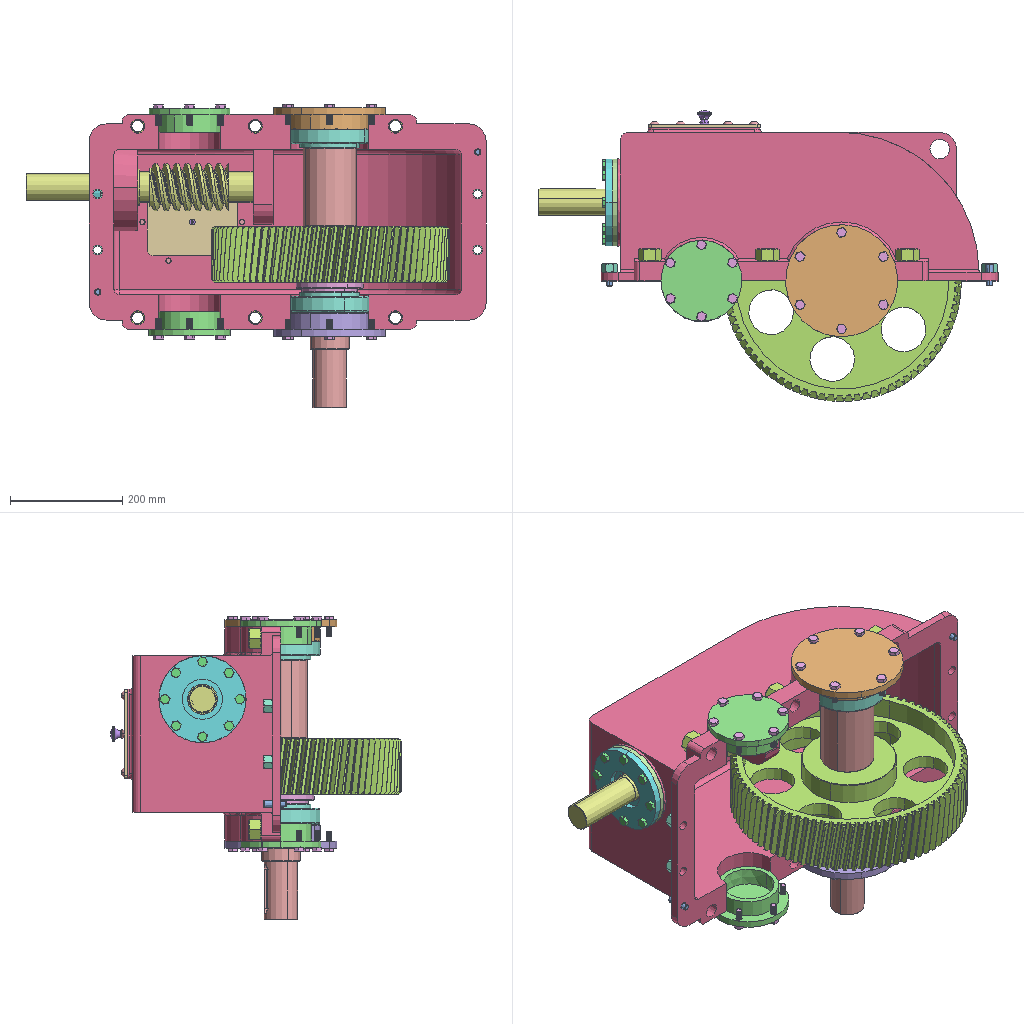Assembly | SolidWorks | 38 different items | 97 placed | box 821 x 519 x 542 mm
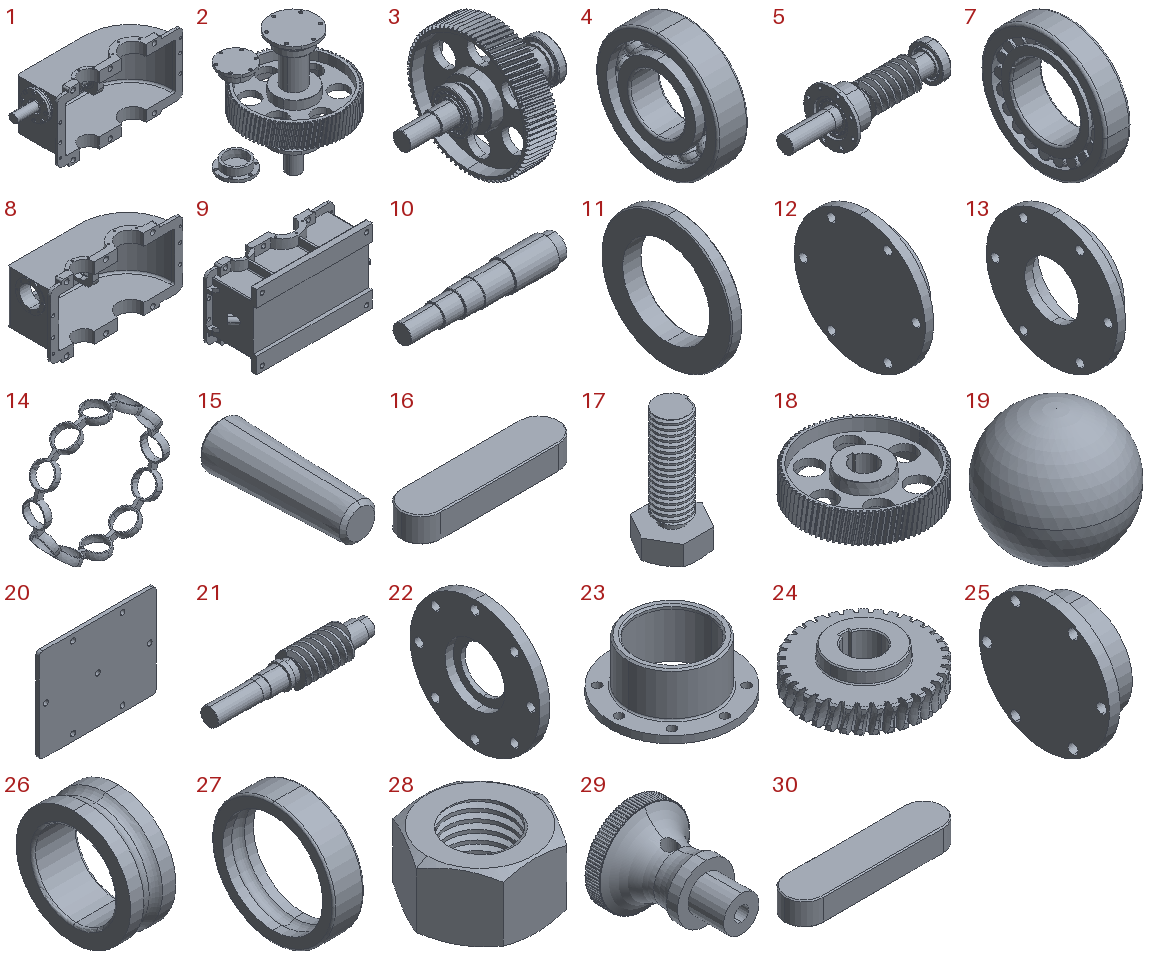Parts list (item | name | quantity | parent item | size | volume | features):
1 | (subassembly) | x1 | - | 820.75 x 304 x 382 mm | 10937552 mm3 | features CompositeCurve 13
2 | (subassembly) | x1 | - | 535.812 x 424.15 x 535.75 mm | 9344461 mm3 | -
3 | (subassembly) | x1 | in 2 | 499.25 x 424.15 x 424.15 mm | 7884570 mm3 | -
4 | (subassembly) | x1 | in 5 | 25 x 100 x 100 mm | 114868 mm3 | features ReferencePattern 11, LocalCirPattern 1
5 | (subassembly) | x1 | in 1 | 432 x 156 x 156 mm | 1680982 mm3 | -
6 | (subassembly) | x1 | - | - | - | -
7 | - | x4 | in 3, 5 | 26.75 x 100 x 100 mm | 98923 mm3 | features Revolution 3, CirPattern 1
8 | - | x1 | in 1 | 708 x 273 x 382 mm | 8807514 mm3 | features ICE 13, Fillet 10, HoleWzd 5, MirrorPattern 4, 3DProfileFeature 2, CirPattern 1, Extrusion 1, RevCut 1, Shell 1
9 | - | x1 | - | 708.739 x 260 x 410 mm | 11835781 mm3 | features ICE 11, MirrorPattern 5, Fillet 4, HoleWzd 4, CirPattern 3, Rib 2, Extrusion 1, LPattern 1
10 | - | x1 | in 3 | 497 x 95 x 95 mm | 2516140 mm3 | features ICE 2, Chamfer 1, Fillet 1, Revolution 1
11 | - | x1 | in 3 | 17.75 x 120 x 120 mm | 86679 mm3 | features Chamfer 1, Revolution 1
12 | - | x1 | in 2 | 38.75 x 200 x 200 mm | 478948 mm3 | features CirPattern 1, Draft 1, ICE 1, Revolution 1
13 | - | x1 | in 2 | 41 x 200 x 200 mm | 411686 mm3 | features ICE 2, CirPattern 1, Draft 1, Revolution 1
14 | - | x1 | in 4 | 76.5 x 15 x 76.5 mm | 1814 mm3 | features CirPattern 2, Extrusion 1, ICE 1, RevCut 1, Revolution 1
15 | - | x2 | - | 12.933 x 40 x 12.933 mm | 4216 mm3 | features Chamfer 1, Revolution 1
16 | - | x1 | in 3 | 87 x 22 x 14 mm | 25271 mm3 | features Chamfer 1, Extrusion 1
17 | - | x24 | - | 18.475 x 16 x 36.4 mm | 3471 mm3 | features RevCut 2, Extrusion 1, Helix 1, ICE 1, SweepCut 1
18 | - | x1 | in 3 | 424.15 x 424.15 x 100 mm | 4768467 mm3 | features ICE 4, Chamfer 2, CirPattern 2, Draft 1, Extrusion 1, Helix 1, SweepCut 1
19 | - | x12 | in 4 | 13.7 x 13.7 x 13.7 mm | 1346 mm3 | features Revolution 1
20 | - | x1 | in 1 | 200 x 6 x 160 mm | 189431 mm3 | features Extrusion 1, Fillet 1, HoleWzd 1
21 | - | x1 | in 5 | 431 x 84 x 84 mm | 1175756 mm3 | features Chamfer 1, CirPattern 1, Fillet 1, Helix 1, ICE 1, Revolution 1, SweepCut 1
22 | - | x1 | in 1 | 18.5 x 156 x 156 mm | 196663 mm3 | features CirPattern 1, ICE 1, Revolution 1
23 | - | x1 | in 5 | 156 x 156 x 65 mm | 192466 mm3 | features ICE 4, Chamfer 1, CirPattern 1, Extrusion 1, Fillet 1
24 | - | x1 | - | 225 x 225 x 90 mm | 1797406 mm3 | features Chamfer 2, ICE 2, CirPattern 1, Extrusion 1, Fillet 1, Helix 1, MirrorPattern 1, RevCut 1, SweepCut 1
25 | - | x2 | in 2 | 43.25 x 145 x 145 mm | 284628 mm3 | features CirPattern 1, Draft 1, ICE 1, Revolution 1
26 | - | x1 | in 4 | 25 x 63.4 x 63.4 mm | 35870 mm3 | features Fillet 1, Revolution 1
27 | - | x1 | in 4 | 25 x 100 x 100 mm | 61028 mm3 | features Fillet 1, Revolution 1
28 | - | x6 | - | 41.569 x 36 x 22 mm | 16274 mm3 | features Extrusion 1, Helix 1, ICE 1, RevCut 1, SweepCut 1
29 | - | x1 | in 1 | 25.5 x 35 x 25.5 mm | 6761 mm3 | features ICE 3, CirPattern 1, Revolution 1
30 | - | x1 | - | 74 x 18 x 11 mm | 13845 mm3 | features Chamfer 1, Extrusion 1
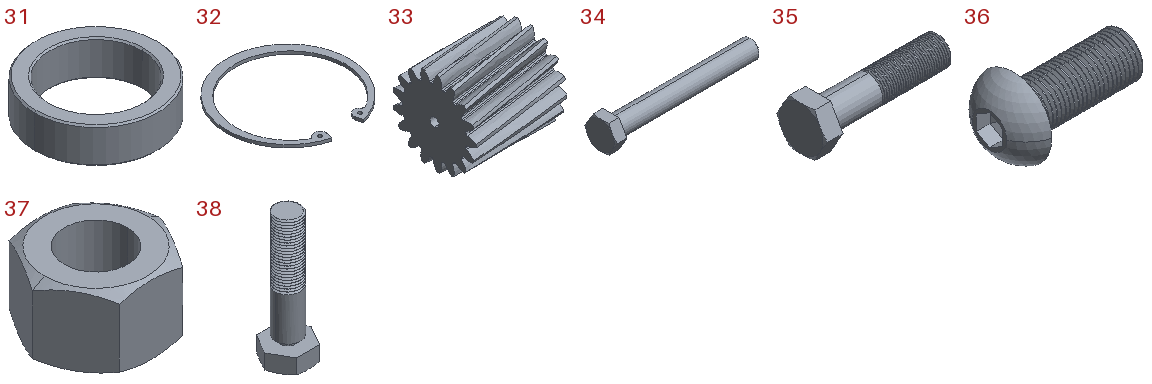31 | - | x1 | - | 80 x 80 x 23 mm | 50140 mm3 | features Chamfer 1, Extrusion 1
32 | - | x1 | in 1 | 105.5 x 103.703 x 2.5 mm | 4495 mm3 | features Extrusion 1
33 | - | x1 | - | 104 x 95.86 x 95.86 mm | 585543 mm3 | features Boss 3, CirPattern 3, Cut 2, Helix 2, SweepCut 2, Revolution 1
34 | - | x1 | - | 97.5 x 20.785 x 18 mm | 12242 mm3 | features RevCut 3, Boss 1, Chamfer 1, Extrusion 1, Fillet 1, LPattern 1
35 | - | x1 | - | 75 x 27.713 x 24 mm | 17249 mm3 | features RevCut 3, Boss 1, Chamfer 1, Extrusion 1, Fillet 1, LPattern 1
36 | - | x6 | in 1 | 30.5 x 17.5 x 17.5 mm | 2529 mm3 | features Cut 2, RevCut 2, Boss 1, Extrusion 1, Fillet 1, LPattern 1
37 | - | x4 | - | 27.713 x 24 x 15.8 mm | 5411 mm3 | features Extrusion 1, ICE 1, RevCut 1
38 | - | x8 | in 1 | 18.475 x 16 x 51.4 mm | 4563 mm3 | features RevCut 2, Extrusion 1, Helix 1, ICE 1, SweepCut 1
Mates (type | each side: item.copy, entity, surface, feature):
In the top assembly
Coincident | assembly face | 8.1 face plane Boss-Extrude2
Concentric | assembly face | 8.1 face cylinder Cut-Extrude3
Concentric | 8.1 face cylinder Cut-Extrude4 | 15.1 face cone Revolve4
DistanceDim | 15.1 face plane Revolve4 | 8.1 face plane Boss-Extrude2
Concentric | 8.1 face cylinder Cut-Extrude4 | 15.2 face cone Revolve4
DistanceDim | 15.2 face plane Revolve4 | 8.1 face plane Boss-Extrude2
Coincident | 8.1 face plane Boss-Extrude5 | 28.1 face plane Boss-Extrude1
Concentric | assembly face | assembly face | 2 times
Parallel | assembly face | assembly face
Coincident | 8.1 face plane Boss-Extrude5 | 28.2 face plane Boss-Extrude1
Coincident | 8.1 face plane Mirror3 | 28.3 face plane Boss-Extrude1
Coincident | 8.1 face plane Mirror3 | 28.4 face plane Boss-Extrude1
Coincident | 8.1 face plane Mirror3 | 28.5 face plane Boss-Extrude1
Concentric | 13.1 face cylinder CirPattern1 | 17.1 face cylinder Cut-Revolve8
Coincident | 13.1 face plane Revolve1 | 17.1 face plane Boss-Extrude1
Concentric | 25.1 face cylinder Cut-Extrude1 | 17.2 face cylinder Cut-Revolve8
Coincident | 25.1 face plane Revolve1 | 17.2 face plane Boss-Extrude1
Concentric | 12.1 face cylinder CirPattern1 | 17.3 face cylinder Cut-Revolve8
Coincident | 12.1 face plane Revolve1 | 17.3 face plane Boss-Extrude1
Concentric | 25.2 face cylinder CirPattern1 | 17.4 face cylinder Cut-Revolve8
Coincident | 25.2 face plane Revolve1 | 17.4 face plane Boss-Extrude1
Coincident | 8.1 face plane Boss-Extrude2 | 37.1 face plane Boss-Extrude1
Coincident | 8.1 face plane Boss-Extrude2 | 37.2 face plane Boss-Extrude1
Coincident | 8.1 face plane Boss-Extrude2 | 37.3 face plane Boss-Extrude1
Coincident | 8.1 face plane Boss-Extrude2 | 37.4 face plane Boss-Extrude1
In subassembly 1
Concentric | 8.2 face cylinder Cut-Extrude2 | 32.1 face cylinder Body
Coincident | 8.2 face plane Cut-Revolve1 | 32.1 face plane Body
Concentric | 8.2 face cylinder Ø1.0 (110) Diameter Hole1 | 23.1 face cylinder Boss-Extrude2
Concentric | 8.2 face cylinder M10 Tapped Hole10 | 23.1 edge
Coincident | 8.2 face plane Boss-Extrude6 | 23.1 face plane Boss-Extrude1
Coincident | 23.1 face plane Boss-Extrude1 | 22.1 face plane Revolve1
Concentric | 21.1 face cylinder Revolve1 | 22.1 face cylinder Revolve1
Concentric | 8.2 face cylinder CirPattern2 | 22.1 face cylinder CirPattern1
Coincident | 8.2 face plane Boss-Extrude9 | 20.1 face plane Boss-Extrude1
Concentric | 8.2 edge | 20.1 edge | 2 times
Concentric | 20.1 face cylinder M10 Tapped Hole1 | 29.1 face cylinder Revolve3
Coincident | 20.1 face plane Boss-Extrude1 | 29.1 edge
Concentric | 22.1 face cylinder Cut-Extrude1 | 38.1 face cylinder Cut-Revolve2
Coincident | 22.1 face plane Revolve1 | 38.1 face plane Boss-Extrude1
Concentric | 22.1 face cylinder CirPattern1 | 38.2 face cylinder Cut-Revolve2
Concentric | 22.1 face cylinder CirPattern1 | 38.3 face cylinder Cut-Revolve2
Concentric | 22.1 edge | 38.4 face cylinder Cut-Revolve2
Concentric | 22.1 face cylinder CirPattern1 | 38.5 face cylinder Cut-Revolve2
Concentric | 22.1 face cylinder CirPattern1 | 38.6 face cylinder Cut-Revolve2
Concentric | 22.1 face cylinder CirPattern1 | 38.7 face cylinder Cut-Revolve2
Concentric | 22.1 face cylinder CirPattern1 | 38.8 face cylinder Cut-Revolve2
Coincident | 22.1 face plane Revolve1 | 38.8 face plane Boss-Extrude1
Coincident | 22.1 face plane Revolve1 | 38.6 face plane Boss-Extrude1
Coincident | 22.1 face plane Revolve1 | 38.7 face plane Boss-Extrude1
Coincident | 22.1 face plane Revolve1 | 38.2 face plane Boss-Extrude1
Coincident | 22.1 face plane Revolve1 | 38.3 face plane Boss-Extrude1
Coincident | 22.1 face plane Revolve1 | 38.4 face plane Boss-Extrude1
Coincident | 22.1 face plane Revolve1 | 38.5 face plane Boss-Extrude1
Concentric | 20.1 face cylinder M10 Tapped Hole1 | 36.1 face cylinder BaseBody
Coincident | 20.1 face plane Boss-Extrude1 | 36.1 face plane BaseHead
Concentric | 20.1 face cylinder M10 Tapped Hole1 | 36.2 face cylinder BaseBody
Coincident | 20.1 face plane Boss-Extrude1 | 36.2 face plane BaseHead
Concentric | 20.1 face cylinder M10 Tapped Hole1 | 36.3 face cylinder BaseBody
Coincident | 20.1 face plane Boss-Extrude1 | 36.3 face plane BaseHead
Concentric | 20.1 face cylinder M10 Tapped Hole1 | 36.4 face cylinder BaseBody
Coincident | 20.1 face plane Boss-Extrude1 | 36.4 face plane BaseHead
Concentric | 20.1 face cylinder M10 Tapped Hole1 | 36.5 face cylinder BaseBody
Coincident | 20.1 face plane Boss-Extrude1 | 36.5 face plane BaseHead
Concentric | 20.1 face cylinder M10 Tapped Hole1 | 36.6 face cylinder BaseBody
Coincident | 20.1 face plane Boss-Extrude1 | 36.6 face plane BaseHead
In subassembly 5
Concentric | 21.2 face cylinder Revolve1 | 26.1 face cylinder Revolve1
Coincident | 21.2 face plane Revolve1 | 26.1 face plane Revolve1
Concentric | 7.1 face cylinder Revolve3 | 7.2 face cylinder Revolve3
Coincident | 7.1 face plane Revolve1 | 7.2 face plane Revolve1
Concentric | 23.2 face cylinder Cut-Extrude2 | 7.2 face cylinder Revolve3
Coincident | 23.2 face plane Cut-Extrude2 | 7.1 face plane Revolve3
Concentric | 21.2 face cylinder Revolve1 | 23.2 face cylinder Boss-Extrude2
Coincident | 21.2 face plane Revolve1 | 7.1 face plane Revolve1
In subassembly 4
Concentric | 26.2 face cylinder Revolve1 | 27.1 face cylinder Revolve1
Coincident | 26.2 face plane Revolve1 | 27.1 face plane Revolve1
Coincident | 27.1 plane | 14.1 plane
Coincident | 26.2 axis | 14.1 axis
Concentric | 19.1 face sphere Revolve1 | 14.1 face sphere CirPattern1
In subassembly 2
Concentric | 7.3 face cylinder Revolve3 | 12.2 face cone Revolve1
Coincident | 7.3 face plane Revolve1 | 12.2 face plane Revolve1
In subassembly 3
Coincident | 10.1 face plane Cut-Extrude2 | 16.1 face plane Boss-Extrude1
Concentric | 10.1 face cylinder Cut-Extrude2 | 16.1 face cylinder Boss-Extrude1
Coincident | 16.1 face plane Boss-Extrude1 | 18.1 face plane Cut-Extrude1 | 2 times
Coincident | 10.1 face plane Revolve2 | 18.1 face plane Boss-Extrude1
Concentric | 10.1 face cylinder Revolve2 | 11.1 face cylinder Revolve1
Coincident | 18.1 face plane Boss-Extrude1 | 11.1 face plane Revolve1
Concentric | 10.1 face cylinder Revolve2 | 7.1 face cylinder Revolve1
Coincident | 11.1 face plane Revolve1 | 7.1 face plane Revolve1
Concentric | 10.1 face cylinder Revolve2 | 7.2 face cylinder Revolve1
Coincident | 10.1 face plane Revolve2 | 7.2 face plane Revolve1